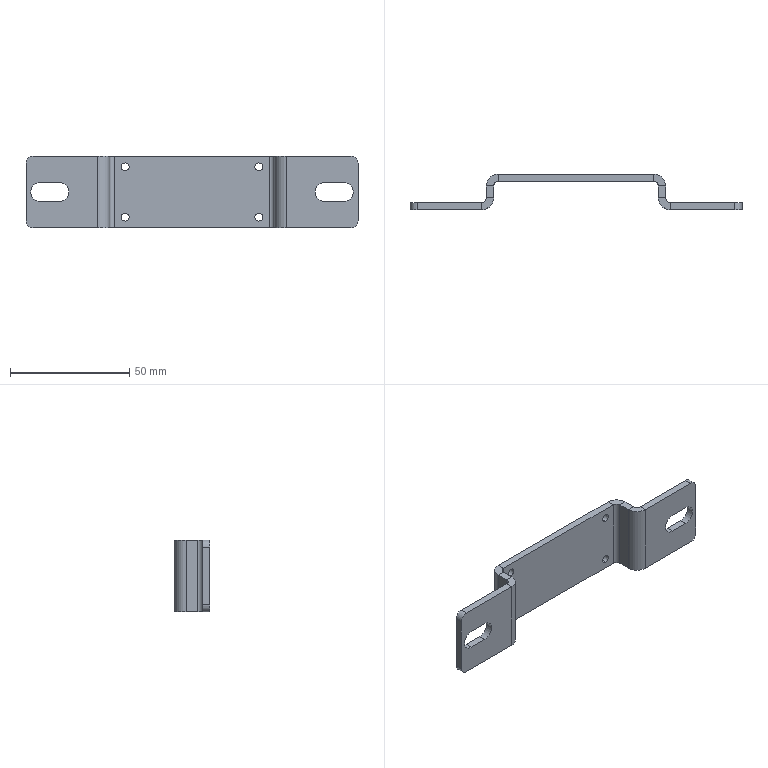Part | SolidWorks | features EdgeFlange 2, Fillet 1, FlatPattern 1, HoleWzd 1, ICE 1, MirrorPattern 1, SMBaseFlange 1, SheetMetal 1 | 1 solid | 58 faces | box 139 x 15 x 30 mm | volume 13318 mm3 | plane 34 | cylinder 24 | commonest cylinder face diameters 3.3 x8 4 x4 6 x4 8 x4 10 x4